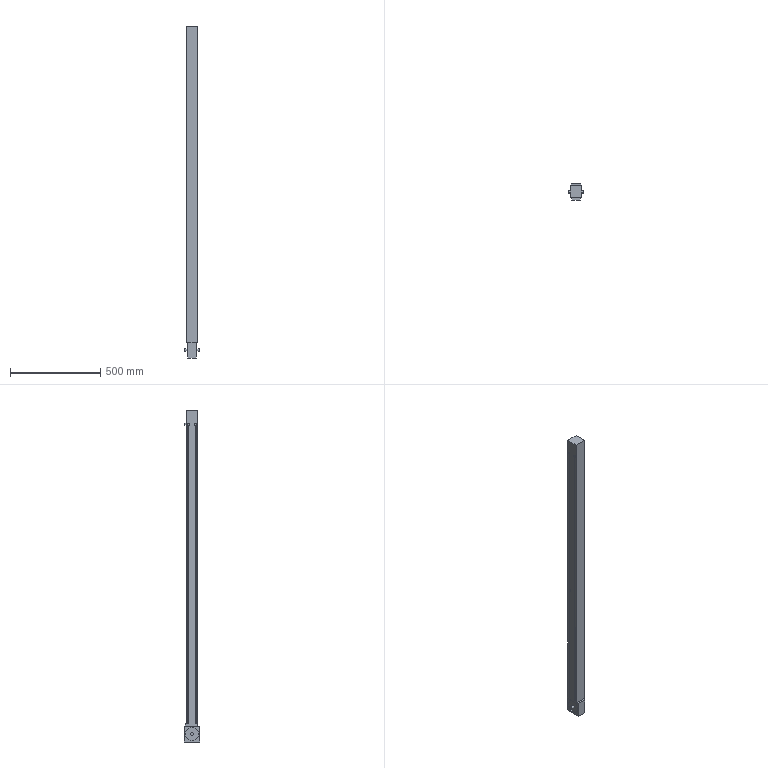Part | SolidWorks | features Boss 5, Cut 2, MirrorPattern 2, Extrusion 1 | 1 solid | 93 faces | box 80 x 88 x 1836 mm | volume 7212179 mm3 | plane 77 | cylinder 16 | commonest cylinder face diameters 8 x8 16 x4 73 x4